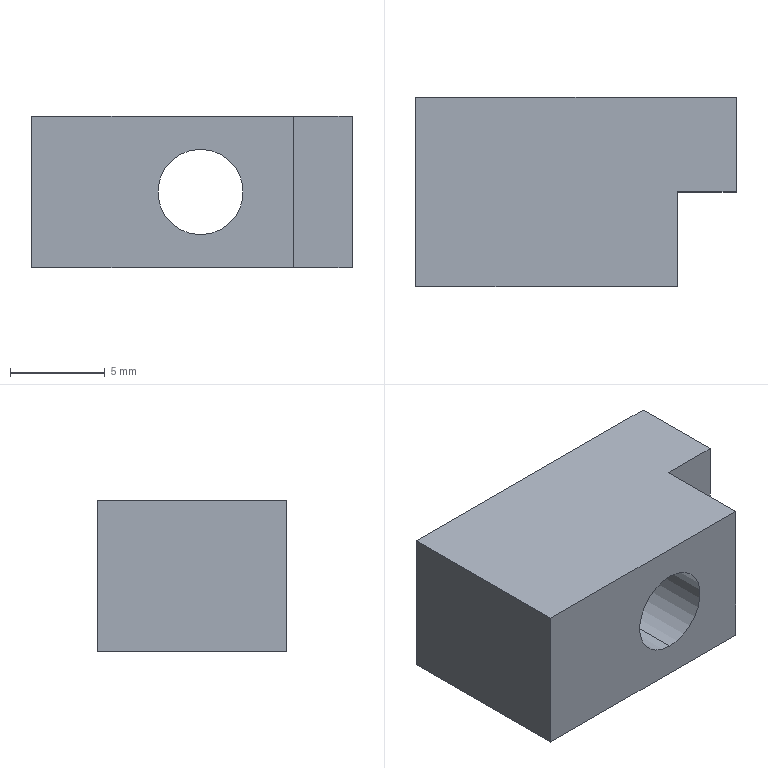Part | STEP file | Shift T-head fixing seat | 1 solid | 13 faces | box 16.9 x 10 x 8 mm | volume 941.722 mm3 | plane 9 | cylinder 4 | commonest cylinder face diameters 4.5 x2 7.5 x2
STEP:
#1=CARTESIAN_POINT('',(0.,0.,0.));
#2=DIRECTION('',(0.,0.,1.));
#3=DIRECTION('',(1.,0.,0.));
#4=AXIS2_PLACEMENT_3D('',#1,#2,#3);
#5=CARTESIAN_POINT('',(4.,5.5,7.75));
#6=VERTEX_POINT('',#5);
#7=CARTESIAN_POINT('',(4.,10.,7.75));
#8=VERTEX_POINT('',#7);
#9=CARTESIAN_POINT('',(4.,10.,7.75));
#10=DIRECTION('',(0.,1.,0.));
#11=VECTOR('',#10,1.);
#12=LINE('',#9,#11);
#13=CARTESIAN_POINT('',(4.,10.,4.));
#14=DIRECTION('',(0.,1.,0.));
#15=DIRECTION('',(0.,0.,1.));
#16=AXIS2_PLACEMENT_3D('',#13,#14,#15);
#17=CYLINDRICAL_SURFACE('',#16,3.75);
#18=CARTESIAN_POINT('',(6.283,0.));
#19=DIRECTION('',(0.,1.));
#20=VECTOR('',#19,1.);
#21=LINE('',#18,#20);
#22=(GEOMETRIC_REPRESENTATION_CONTEXT(2)PARAMETRIC_REPRESENTATION_CONTEXT()REPRESENTATION_CONTEXT('',''));
#23=DEFINITIONAL_REPRESENTATION('',(#21),#22);
#24=PCURVE('',#17,#23);
#25=CARTESIAN_POINT('',(4.,10.,4.));
#26=DIRECTION('',(0.,1.,0.));
#27=DIRECTION('',(0.,0.,1.));
#28=AXIS2_PLACEMENT_3D('',#25,#26,#27);
#29=CYLINDRICAL_SURFACE('',#28,3.75);
#30=CARTESIAN_POINT('',(0.,0.));
#31=DIRECTION('',(0.,1.));
#32=VECTOR('',#31,1.);
#33=LINE('',#30,#32);
#34=(GEOMETRIC_REPRESENTATION_CONTEXT(2)PARAMETRIC_REPRESENTATION_CONTEXT()REPRESENTATION_CONTEXT('',''));
#35=DEFINITIONAL_REPRESENTATION('',(#33),#34);
#36=PCURVE('',#29,#35);
#37=SURFACE_CURVE('',#12,(#24,#36),.PCURVE_S1.);
#38=EDGE_CURVE('',#6,#8,#37,.T.);
#39=ORIENTED_EDGE('',*,*,#38,.T.);
#40=CARTESIAN_POINT('',(4.,10.,0.25));
#41=VERTEX_POINT('',#40);
#42=CARTESIAN_POINT('',(4.,10.,4.));
#43=DIRECTION('',(0.,1.,0.));
#44=DIRECTION('',(0.,0.,1.));
#45=AXIS2_PLACEMENT_3D('',#42,#43,#44);
#46=CIRCLE('',#45,3.75);
#47=CARTESIAN_POINT('',(0.,0.));
#48=DIRECTION('',(1.,0.));
#49=VECTOR('',#48,1.);
#50=LINE('',#47,#49);
#51=(GEOMETRIC_REPRESENTATION_CONTEXT(2)PARAMETRIC_REPRESENTATION_CONTEXT()REPRESENTATION_CONTEXT('',''));
#52=DEFINITIONAL_REPRESENTATION('',(#50),#51);
#53=PCURVE('',#17,#52);
#54=CARTESIAN_POINT('',(0.,10.,8.));
#55=DIRECTION('',(0.,-1.,0.));
#56=DIRECTION('',(1.,0.,0.));
#57=AXIS2_PLACEMENT_3D('',#54,#55,#56);
#58=PLANE('',#57);
#59=CARTESIAN_POINT('',(4.,-0.25));
#60=CARTESIAN_POINT('',(10.495,-0.25));
#61=CARTESIAN_POINT('',(7.248,-5.875));
#62=CARTESIAN_POINT('',(4.,-11.5));
#63=CARTESIAN_POINT('',(0.7524,-5.875));
#64=CARTESIAN_POINT('',(-2.495,-0.25));
#65=CARTESIAN_POINT('',(4.,-0.25));
#66=(BOUNDED_CURVE()B_SPLINE_CURVE(2,(#59,#60,#61,#62,#63,#64,#65),.UNSPECIFIED.,.T.,.F.)B_SPLINE_CURVE_WITH_KNOTS((1,2,2,2,2,1),(-2.094,0.,2.094,4.189,6.283,8.378),.UNSPECIFIED.)CURVE()GEOMETRIC_REPRESENTATION_ITEM()RATIONAL_B_SPLINE_CURVE((1.,0.5,1.,0.5,1.,0.5,1.))REPRESENTATION_ITEM(''));
#67=(GEOMETRIC_REPRESENTATION_CONTEXT(2)PARAMETRIC_REPRESENTATION_CONTEXT()REPRESENTATION_CONTEXT('',''));
#68=DEFINITIONAL_REPRESENTATION('',(#66),#67);
#69=PCURVE('',#58,#68);
#70=SURFACE_CURVE('',#46,(#53,#69),.PCURVE_S1.);
#71=EDGE_CURVE('',#41,#8,#70,.T.);
#72=ORIENTED_EDGE('',*,*,#71,.F.);
#73=CARTESIAN_POINT('',(4.,5.5,0.25));
#74=VERTEX_POINT('',#73);
#75=CARTESIAN_POINT('',(4.,10.,0.25));
#76=DIRECTION('',(0.,1.,0.));
#77=VECTOR('',#76,1.);
#78=LINE('',#75,#77);
#79=CARTESIAN_POINT('',(3.142,0.));
#80=DIRECTION('',(0.,1.));
#81=VECTOR('',#80,1.);
#82=LINE('',#79,#81);
#83=(GEOMETRIC_REPRESENTATION_CONTEXT(2)PARAMETRIC_REPRESENTATION_CONTEXT()REPRESENTATION_CONTEXT('',''));
#84=DEFINITIONAL_REPRESENTATION('',(#82),#83);
#85=PCURVE('',#17,#84);
#86=CARTESIAN_POINT('',(3.142,0.));
#87=DIRECTION('',(0.,1.));
#88=VECTOR('',#87,1.);
#89=LINE('',#86,#88);
#90=(GEOMETRIC_REPRESENTATION_CONTEXT(2)PARAMETRIC_REPRESENTATION_CONTEXT()REPRESENTATION_CONTEXT('',''));
#91=DEFINITIONAL_REPRESENTATION('',(#89),#90);
#92=PCURVE('',#29,#91);
#93=SURFACE_CURVE('',#78,(#85,#92),.PCURVE_S1.);
#94=EDGE_CURVE('',#74,#41,#93,.T.);
#95=ORIENTED_EDGE('',*,*,#94,.F.);
#96=CARTESIAN_POINT('',(4.,5.5,4.));
#97=DIRECTION('',(0.,1.,0.));
#98=DIRECTION('',(0.,0.,1.));
#99=AXIS2_PLACEMENT_3D('',#96,#97,#98);
#100=CIRCLE('',#99,3.75);
#101=CARTESIAN_POINT('',(0.,-4.5));
#102=DIRECTION('',(1.,0.));
#103=VECTOR('',#102,1.);
#104=LINE('',#101,#103);
#105=(GEOMETRIC_REPRESENTATION_CONTEXT(2)PARAMETRIC_REPRESENTATION_CONTEXT()REPRESENTATION_CONTEXT('',''));
#106=DEFINITIONAL_REPRESENTATION('',(#104),#105);
#107=PCURVE('',#17,#106);
#108=CARTESIAN_POINT('',(6.25,5.5,4.));
#109=DIRECTION('',(0.,-1.,0.));
#110=DIRECTION('',(0.,0.,-1.));
#111=AXIS2_PLACEMENT_3D('',#108,#109,#110);
#112=PLANE('',#111);
#113=CARTESIAN_POINT('',(-3.75,-2.25));
#114=CARTESIAN_POINT('',(-3.75,4.245));
#115=CARTESIAN_POINT('',(1.875,0.9976));
#116=CARTESIAN_POINT('',(7.5,-2.25));
#117=CARTESIAN_POINT('',(1.875,-5.498));
#118=CARTESIAN_POINT('',(-3.75,-8.745));
#119=CARTESIAN_POINT('',(-3.75,-2.25));
#120=(BOUNDED_CURVE()B_SPLINE_CURVE(2,(#113,#114,#115,#116,#117,#118,#119),.UNSPECIFIED.,.T.,.F.)B_SPLINE_CURVE_WITH_KNOTS((1,2,2,2,2,1),(-2.094,0.,2.094,4.189,6.283,8.378),.UNSPECIFIED.)CURVE()GEOMETRIC_REPRESENTATION_ITEM()RATIONAL_B_SPLINE_CURVE((1.,0.5,1.,0.5,1.,0.5,1.))REPRESENTATION_ITEM(''));
#121=(GEOMETRIC_REPRESENTATION_CONTEXT(2)PARAMETRIC_REPRESENTATION_CONTEXT()REPRESENTATION_CONTEXT('',''));
#122=DEFINITIONAL_REPRESENTATION('',(#120),#121);
#123=PCURVE('',#112,#122);
#124=SURFACE_CURVE('',#100,(#107,#123),.PCURVE_S1.);
#125=EDGE_CURVE('',#74,#6,#124,.T.);
#126=ORIENTED_EDGE('',*,*,#125,.T.);
#127=EDGE_LOOP('',(#39,#72,#95,#126));
#128=FACE_BOUND('',#127,.F.);
#129=ADVANCED_FACE('',(#128),#17,.F.);
#130=CARTESIAN_POINT('',(4.,0.,6.25));
#131=VERTEX_POINT('',#130);
#132=CARTESIAN_POINT('',(4.,5.5,6.25));
#133=VERTEX_POINT('',#132);
#134=CARTESIAN_POINT('',(4.,10.,6.25));
#135=DIRECTION('',(0.,1.,0.));
#136=VECTOR('',#135,1.);
#137=LINE('',#134,#136);
#138=CARTESIAN_POINT('',(4.,10.,4.));
#139=DIRECTION('',(0.,1.,0.));
#140=DIRECTION('',(0.,0.,1.));
#141=AXIS2_PLACEMENT_3D('',#138,#139,#140);
#142=CYLINDRICAL_SURFACE('',#141,2.25);
#143=CARTESIAN_POINT('',(6.283,0.));
#144=DIRECTION('',(0.,1.));
#145=VECTOR('',#144,1.);
#146=LINE('',#143,#145);
#147=(GEOMETRIC_REPRESENTATION_CONTEXT(2)PARAMETRIC_REPRESENTATION_CONTEXT()REPRESENTATION_CONTEXT('',''));
#148=DEFINITIONAL_REPRESENTATION('',(#146),#147);
#149=PCURVE('',#142,#148);
#150=CARTESIAN_POINT('',(4.,10.,4.));
#151=DIRECTION('',(0.,1.,0.));
#152=DIRECTION('',(0.,0.,1.));
#153=AXIS2_PLACEMENT_3D('',#150,#151,#152);
#154=CYLINDRICAL_SURFACE('',#153,2.25);
#155=CARTESIAN_POINT('',(0.,0.));
#156=DIRECTION('',(0.,1.));
#157=VECTOR('',#156,1.);
#158=LINE('',#155,#157);
#159=(GEOMETRIC_REPRESENTATION_CONTEXT(2)PARAMETRIC_REPRESENTATION_CONTEXT()REPRESENTATION_CONTEXT('',''));
#160=DEFINITIONAL_REPRESENTATION('',(#158),#159);
#161=PCURVE('',#154,#160);
#162=SURFACE_CURVE('',#137,(#149,#161),.PCURVE_S1.);
#163=EDGE_CURVE('',#131,#133,#162,.T.);
#164=ORIENTED_EDGE('',*,*,#163,.T.);
#165=CARTESIAN_POINT('',(4.,5.5,1.75));
#166=VERTEX_POINT('',#165);
#167=CARTESIAN_POINT('',(4.,5.5,4.));
#168=DIRECTION('',(0.,1.,0.));
#169=DIRECTION('',(0.,0.,1.));
#170=AXIS2_PLACEMENT_3D('',#167,#168,#169);
#171=CIRCLE('',#170,2.25);
#172=CARTESIAN_POINT('',(0.,-4.5));
#173=DIRECTION('',(1.,0.));
#174=VECTOR('',#173,1.);
#175=LINE('',#172,#174);
#176=(GEOMETRIC_REPRESENTATION_CONTEXT(2)PARAMETRIC_REPRESENTATION_CONTEXT()REPRESENTATION_CONTEXT('',''));
#177=DEFINITIONAL_REPRESENTATION('',(#175),#176);
#178=PCURVE('',#142,#177);
#179=CARTESIAN_POINT('',(-2.25,-2.25));
#180=CARTESIAN_POINT('',(-2.25,1.647));
#181=CARTESIAN_POINT('',(1.125,-0.3014));
#182=CARTESIAN_POINT('',(4.5,-2.25));
#183=CARTESIAN_POINT('',(1.125,-4.199));
#184=CARTESIAN_POINT('',(-2.25,-6.147));
#185=CARTESIAN_POINT('',(-2.25,-2.25));
#186=(BOUNDED_CURVE()B_SPLINE_CURVE(2,(#179,#180,#181,#182,#183,#184,#185),.UNSPECIFIED.,.T.,.F.)B_SPLINE_CURVE_WITH_KNOTS((1,2,2,2,2,1),(-2.094,0.,2.094,4.189,6.283,8.378),.UNSPECIFIED.)CURVE()GEOMETRIC_REPRESENTATION_ITEM()RATIONAL_B_SPLINE_CURVE((1.,0.5,1.,0.5,1.,0.5,1.))REPRESENTATION_ITEM(''));
#187=(GEOMETRIC_REPRESENTATION_CONTEXT(2)PARAMETRIC_REPRESENTATION_CONTEXT()REPRESENTATION_CONTEXT('',''));
#188=DEFINITIONAL_REPRESENTATION('',(#186),#187);
#189=PCURVE('',#112,#188);
#190=SURFACE_CURVE('',#171,(#178,#189),.PCURVE_S1.);
#191=EDGE_CURVE('',#166,#133,#190,.T.);
#192=ORIENTED_EDGE('',*,*,#191,.F.);
#193=CARTESIAN_POINT('',(4.,0.,1.75));
#194=VERTEX_POINT('',#193);
#195=CARTESIAN_POINT('',(4.,10.,1.75));
#196=DIRECTION('',(0.,1.,0.));
#197=VECTOR('',#196,1.);
#198=LINE('',#195,#197);
#199=CARTESIAN_POINT('',(3.142,0.));
#200=DIRECTION('',(0.,1.));
#201=VECTOR('',#200,1.);
#202=LINE('',#199,#201);
#203=(GEOMETRIC_REPRESENTATION_CONTEXT(2)PARAMETRIC_REPRESENTATION_CONTEXT()REPRESENTATION_CONTEXT('',''));
#204=DEFINITIONAL_REPRESENTATION('',(#202),#203);
#205=PCURVE('',#142,#204);
#206=CARTESIAN_POINT('',(3.142,0.));
#207=DIRECTION('',(0.,1.));
#208=VECTOR('',#207,1.);
#209=LINE('',#206,#208);
#210=(GEOMETRIC_REPRESENTATION_CONTEXT(2)PARAMETRIC_REPRESENTATION_CONTEXT()REPRESENTATION_CONTEXT('',''));
#211=DEFINITIONAL_REPRESENTATION('',(#209),#210);
#212=PCURVE('',#154,#211);
#213=SURFACE_CURVE('',#198,(#205,#212),.PCURVE_S1.);
#214=EDGE_CURVE('',#194,#166,#213,.T.);
#215=ORIENTED_EDGE('',*,*,#214,.F.);
#216=CARTESIAN_POINT('',(4.,0.,4.));
#217=DIRECTION('',(0.,1.,0.));
#218=DIRECTION('',(0.,0.,1.));
#219=AXIS2_PLACEMENT_3D('',#216,#217,#218);
#220=CIRCLE('',#219,2.25);
#221=CARTESIAN_POINT('',(0.,-10.));
#222=DIRECTION('',(1.,0.));
#223=VECTOR('',#222,1.);
#224=LINE('',#221,#223);
#225=(GEOMETRIC_REPRESENTATION_CONTEXT(2)PARAMETRIC_REPRESENTATION_CONTEXT()REPRESENTATION_CONTEXT('',''));
#226=DEFINITIONAL_REPRESENTATION('',(#224),#225);
#227=PCURVE('',#142,#226);
#228=CARTESIAN_POINT('',(0.,0.,8.));
#229=DIRECTION('',(0.,1.,0.));
#230=DIRECTION('',(0.,0.,1.));
#231=AXIS2_PLACEMENT_3D('',#228,#229,#230);
#232=PLANE('',#231);
#233=CARTESIAN_POINT('',(-4.,4.));
#234=DIRECTION('',(1.,0.));
#235=AXIS2_PLACEMENT_2D('',#233,#234);
#236=CIRCLE('',#235,2.25);
#237=(GEOMETRIC_REPRESENTATION_CONTEXT(2)PARAMETRIC_REPRESENTATION_CONTEXT()REPRESENTATION_CONTEXT('',''));
#238=DEFINITIONAL_REPRESENTATION('',(#236),#237);
#239=PCURVE('',#232,#238);
#240=SURFACE_CURVE('',#220,(#227,#239),.PCURVE_S1.);
#241=EDGE_CURVE('',#194,#131,#240,.T.);
#242=ORIENTED_EDGE('',*,*,#241,.T.);
#243=EDGE_LOOP('',(#164,#192,#215,#242));
#244=FACE_BOUND('',#243,.F.);
#245=ADVANCED_FACE('',(#244),#142,.F.);
#246=CARTESIAN_POINT('',(-4.9,10.,0.));
#247=VERTEX_POINT('',#246);
#248=CARTESIAN_POINT('',(-4.9,0.,0.));
#249=VERTEX_POINT('',#248);
#250=CARTESIAN_POINT('',(-4.9,10.,0.));
#251=DIRECTION('',(0.,-1.,0.));
#252=VECTOR('',#251,1.);
#253=LINE('',#250,#252);
#254=CARTESIAN_POINT('',(-4.9,0.,8.));
#255=DIRECTION('',(1.,0.,0.));
#256=DIRECTION('',(0.,0.,-1.));
#257=AXIS2_PLACEMENT_3D('',#254,#255,#256);
#258=PLANE('',#257);
#259=CARTESIAN_POINT('',(8.,10.));
#260=DIRECTION('',(0.,-1.));
#261=VECTOR('',#260,1.);
#262=LINE('',#259,#261);
#263=(GEOMETRIC_REPRESENTATION_CONTEXT(2)PARAMETRIC_REPRESENTATION_CONTEXT()REPRESENTATION_CONTEXT('',''));
#264=DEFINITIONAL_REPRESENTATION('',(#262),#263);
#265=PCURVE('',#258,#264);
#266=CARTESIAN_POINT('',(0.,10.,0.));
#267=DIRECTION('',(0.,0.,-1.));
#268=DIRECTION('',(-1.,0.,0.));
#269=AXIS2_PLACEMENT_3D('',#266,#267,#268);
#270=PLANE('',#269);
#271=CARTESIAN_POINT('',(4.9,0.));
#272=DIRECTION('',(0.,-1.));
#273=VECTOR('',#272,1.);
#274=LINE('',#271,#273);
#275=(GEOMETRIC_REPRESENTATION_CONTEXT(2)PARAMETRIC_REPRESENTATION_CONTEXT()REPRESENTATION_CONTEXT('',''));
#276=DEFINITIONAL_REPRESENTATION('',(#274),#275);
#277=PCURVE('',#270,#276);
#278=SURFACE_CURVE('',#253,(#265,#277),.PCURVE_S1.);
#279=EDGE_CURVE('',#247,#249,#278,.T.);
#280=ORIENTED_EDGE('',*,*,#279,.T.);
#281=CARTESIAN_POINT('',(-4.9,0.,8.));
#282=VERTEX_POINT('',#281);
#283=CARTESIAN_POINT('',(-4.9,0.,8.));
#284=DIRECTION('',(0.,0.,-1.));
#285=VECTOR('',#284,1.);
#286=LINE('',#283,#285);
#287=CARTESIAN_POINT('',(0.,0.));
#288=DIRECTION('',(1.,0.));
#289=VECTOR('',#288,1.);
#290=LINE('',#287,#289);
#291=(GEOMETRIC_REPRESENTATION_CONTEXT(2)PARAMETRIC_REPRESENTATION_CONTEXT()REPRESENTATION_CONTEXT('',''));
#292=DEFINITIONAL_REPRESENTATION('',(#290),#291);
#293=PCURVE('',#258,#292);
#294=CARTESIAN_POINT('',(0.,-4.9));
#295=DIRECTION('',(-1.,0.));
#296=VECTOR('',#295,1.);
#297=LINE('',#294,#296);
#298=(GEOMETRIC_REPRESENTATION_CONTEXT(2)PARAMETRIC_REPRESENTATION_CONTEXT()REPRESENTATION_CONTEXT('',''));
#299=DEFINITIONAL_REPRESENTATION('',(#297),#298);
#300=PCURVE('',#232,#299);
#301=SURFACE_CURVE('',#286,(#293,#300),.PCURVE_S1.);
#302=EDGE_CURVE('',#282,#249,#301,.T.);
#303=ORIENTED_EDGE('',*,*,#302,.F.);
#304=CARTESIAN_POINT('',(-4.9,10.,8.));
#305=VERTEX_POINT('',#304);
#306=CARTESIAN_POINT('',(-4.9,10.,8.));
#307=DIRECTION('',(0.,-1.,0.));
#308=VECTOR('',#307,1.);
#309=LINE('',#306,#308);
#310=CARTESIAN_POINT('',(0.,10.));
#311=DIRECTION('',(0.,-1.));
#312=VECTOR('',#311,1.);
#313=LINE('',#310,#312);
#314=(GEOMETRIC_REPRESENTATION_CONTEXT(2)PARAMETRIC_REPRESENTATION_CONTEXT()REPRESENTATION_CONTEXT('',''));
#315=DEFINITIONAL_REPRESENTATION('',(#313),#314);
#316=PCURVE('',#258,#315);
#317=CARTESIAN_POINT('',(0.,10.,8.));
#318=DIRECTION('',(0.,0.,-1.));
#319=DIRECTION('',(-1.,0.,0.));
#320=AXIS2_PLACEMENT_3D('',#317,#318,#319);
#321=PLANE('',#320);
#322=CARTESIAN_POINT('',(4.9,0.));
#323=DIRECTION('',(0.,-1.));
#324=VECTOR('',#323,1.);
#325=LINE('',#322,#324);
#326=(GEOMETRIC_REPRESENTATION_CONTEXT(2)PARAMETRIC_REPRESENTATION_CONTEXT()REPRESENTATION_CONTEXT('',''));
#327=DEFINITIONAL_REPRESENTATION('',(#325),#326);
#328=PCURVE('',#321,#327);
#329=SURFACE_CURVE('',#309,(#316,#328),.PCURVE_S1.);
#330=EDGE_CURVE('',#305,#282,#329,.T.);
#331=ORIENTED_EDGE('',*,*,#330,.F.);
#332=CARTESIAN_POINT('',(-4.9,10.,8.));
#333=DIRECTION('',(0.,0.,-1.));
#334=VECTOR('',#333,1.);
#335=LINE('',#332,#334);
#336=CARTESIAN_POINT('',(0.,10.));
#337=DIRECTION('',(1.,0.));
#338=VECTOR('',#337,1.);
#339=LINE('',#336,#338);
#340=(GEOMETRIC_REPRESENTATION_CONTEXT(2)PARAMETRIC_REPRESENTATION_CONTEXT()REPRESENTATION_CONTEXT('',''));
#341=DEFINITIONAL_REPRESENTATION('',(#339),#340);
#342=PCURVE('',#258,#341);
#343=CARTESIAN_POINT('',(-4.9,0.));
#344=DIRECTION('',(0.,-1.));
#345=VECTOR('',#344,1.);
#346=LINE('',#343,#345);
#347=(GEOMETRIC_REPRESENTATION_CONTEXT(2)PARAMETRIC_REPRESENTATION_CONTEXT()REPRESENTATION_CONTEXT('',''));
#348=DEFINITIONAL_REPRESENTATION('',(#346),#347);
#349=PCURVE('',#58,#348);
#350=SURFACE_CURVE('',#335,(#342,#349),.PCURVE_S1.);
#351=EDGE_CURVE('',#305,#247,#350,.T.);
#352=ORIENTED_EDGE('',*,*,#351,.T.);
#353=EDGE_LOOP('',(#280,#303,#331,#352));
#354=FACE_BOUND('',#353,.T.);
#355=ADVANCED_FACE('',(#354),#258,.F.);
#356=CARTESIAN_POINT('',(4.,0.,4.));
#357=DIRECTION('',(0.,1.,0.));
#358=DIRECTION('',(0.,0.,1.));
#359=AXIS2_PLACEMENT_3D('',#356,#357,#358);
#360=CIRCLE('',#359,2.25);
#361=CARTESIAN_POINT('',(-4.,4.));
#362=DIRECTION('',(1.,0.));
#363=AXIS2_PLACEMENT_2D('',#361,#362);
#364=CIRCLE('',#363,2.25);
#365=(GEOMETRIC_REPRESENTATION_CONTEXT(2)PARAMETRIC_REPRESENTATION_CONTEXT()REPRESENTATION_CONTEXT('',''));
#366=DEFINITIONAL_REPRESENTATION('',(#364),#365);
#367=PCURVE('',#232,#366);
#368=CARTESIAN_POINT('',(0.,-10.));
#369=DIRECTION('',(1.,0.));
#370=VECTOR('',#369,1.);
#371=LINE('',#368,#370);
#372=(GEOMETRIC_REPRESENTATION_CONTEXT(2)PARAMETRIC_REPRESENTATION_CONTEXT()REPRESENTATION_CONTEXT('',''));
#373=DEFINITIONAL_REPRESENTATION('',(#371),#372);
#374=PCURVE('',#154,#373);
#375=SURFACE_CURVE('',#360,(#367,#374),.PCURVE_S1.);
#376=EDGE_CURVE('',#131,#194,#375,.T.);
#377=ORIENTED_EDGE('',*,*,#376,.T.);
#378=ORIENTED_EDGE('',*,*,#241,.T.);
#379=EDGE_LOOP('',(#377,#378));
#380=FACE_BOUND('',#379,.T.);
#381=CARTESIAN_POINT('',(8.9,0.,0.));
#382=VERTEX_POINT('',#381);
#383=CARTESIAN_POINT('',(0.,0.,0.));
#384=DIRECTION('',(1.,0.,0.));
#385=VECTOR('',#384,1.);
#386=LINE('',#383,#385);
#387=CARTESIAN_POINT('',(-8.,0.));
#388=DIRECTION('',(0.,1.));
#389=VECTOR('',#388,1.);
#390=LINE('',#387,#389);
#391=(GEOMETRIC_REPRESENTATION_CONTEXT(2)PARAMETRIC_REPRESENTATION_CONTEXT()REPRESENTATION_CONTEXT('',''));
#392=DEFINITIONAL_REPRESENTATION('',(#390),#391);
#393=PCURVE('',#232,#392);
#394=CARTESIAN_POINT('',(0.,-10.));
#395=DIRECTION('',(-1.,0.));
#396=VECTOR('',#395,1.);
#397=LINE('',#394,#396);
#398=(GEOMETRIC_REPRESENTATION_CONTEXT(2)PARAMETRIC_REPRESENTATION_CONTEXT()REPRESENTATION_CONTEXT('',''));
#399=DEFINITIONAL_REPRESENTATION('',(#397),#398);
#400=PCURVE('',#270,#399);
#401=SURFACE_CURVE('',#386,(#393,#400),.PCURVE_S1.);
#402=EDGE_CURVE('',#249,#382,#401,.T.);
#403=ORIENTED_EDGE('',*,*,#402,.T.);
#404=CARTESIAN_POINT('',(8.9,0.,8.));
#405=VERTEX_POINT('',#404);
#406=CARTESIAN_POINT('',(8.9,0.,8.));
#407=DIRECTION('',(0.,0.,1.));
#408=VECTOR('',#407,1.);
#409=LINE('',#406,#408);
#410=CARTESIAN_POINT('',(0.,8.9));
#411=DIRECTION('',(1.,0.));
#412=VECTOR('',#411,1.);
#413=LINE('',#410,#412);
#414=(GEOMETRIC_REPRESENTATION_CONTEXT(2)PARAMETRIC_REPRESENTATION_CONTEXT()REPRESENTATION_CONTEXT('',''));
#415=DEFINITIONAL_REPRESENTATION('',(#413),#414);
#416=PCURVE('',#232,#415);
#417=CARTESIAN_POINT('',(8.9,5.,0.));
#418=DIRECTION('',(-1.,0.,0.));
#419=DIRECTION('',(0.,-1.,0.));
#420=AXIS2_PLACEMENT_3D('',#417,#418,#419);
#421=PLANE('',#420);
#422=CARTESIAN_POINT('',(5.,8.));
#423=DIRECTION('',(0.,1.));
#424=VECTOR('',#423,1.);
#425=LINE('',#422,#424);
#426=(GEOMETRIC_REPRESENTATION_CONTEXT(2)PARAMETRIC_REPRESENTATION_CONTEXT()REPRESENTATION_CONTEXT('',''));
#427=DEFINITIONAL_REPRESENTATION('',(#425),#426);
#428=PCURVE('',#421,#427);
#429=SURFACE_CURVE('',#409,(#416,#428),.PCURVE_S1.);
#430=EDGE_CURVE('',#382,#405,#429,.T.);
#431=ORIENTED_EDGE('',*,*,#430,.T.);
#432=CARTESIAN_POINT('',(0.,0.,8.));
#433=DIRECTION('',(1.,0.,0.));
#434=VECTOR('',#433,1.);
#435=LINE('',#432,#434);
#436=CARTESIAN_POINT('',(0.,0.));
#437=DIRECTION('',(0.,1.));
#438=VECTOR('',#437,1.);
#439=LINE('',#436,#438);
#440=(GEOMETRIC_REPRESENTATION_CONTEXT(2)PARAMETRIC_REPRESENTATION_CONTEXT()REPRESENTATION_CONTEXT('',''));
#441=DEFINITIONAL_REPRESENTATION('',(#439),#440);
#442=PCURVE('',#232,#441);
#443=CARTESIAN_POINT('',(0.,-10.));
#444=DIRECTION('',(-1.,0.));
#445=VECTOR('',#444,1.);
#446=LINE('',#443,#445);
#447=(GEOMETRIC_REPRESENTATION_CONTEXT(2)PARAMETRIC_REPRESENTATION_CONTEXT()REPRESENTATION_CONTEXT('',''));
#448=DEFINITIONAL_REPRESENTATION('',(#446),#447);
#449=PCURVE('',#321,#448);
#450=SURFACE_CURVE('',#435,(#442,#449),.PCURVE_S1.);
#451=EDGE_CURVE('',#282,#405,#450,.T.);
#452=ORIENTED_EDGE('',*,*,#451,.F.);
#453=ORIENTED_EDGE('',*,*,#302,.T.);
#454=EDGE_LOOP('',(#403,#431,#452,#453));
#455=FACE_BOUND('',#454,.T.);
#456=ADVANCED_FACE('',(#380,#455),#232,.F.);
#457=CARTESIAN_POINT('',(12.,5.,8.));
#458=VERTEX_POINT('',#457);
#459=CARTESIAN_POINT('',(12.,10.,8.));
#460=VERTEX_POINT('',#459);
#461=CARTESIAN_POINT('',(12.,0.,8.));
#462=DIRECTION('',(0.,1.,0.));
#463=VECTOR('',#462,1.);
#464=LINE('',#461,#463);
#465=CARTESIAN_POINT('',(12.,0.,8.));
#466=DIRECTION('',(-1.,0.,0.));
#467=DIRECTION('',(0.,0.,1.));
#468=AXIS2_PLACEMENT_3D('',#465,#466,#467);
#469=PLANE('',#468);
#470=CARTESIAN_POINT('',(0.,0.));
#471=DIRECTION('',(0.,1.));
#472=VECTOR('',#471,1.);
#473=LINE('',#470,#472);
#474=(GEOMETRIC_REPRESENTATION_CONTEXT(2)PARAMETRIC_REPRESENTATION_CONTEXT()REPRESENTATION_CONTEXT('',''));
#475=DEFINITIONAL_REPRESENTATION('',(#473),#474);
#476=PCURVE('',#469,#475);
#477=CARTESIAN_POINT('',(-12.,-10.));
#478=DIRECTION('',(0.,1.));
#479=VECTOR('',#478,1.);
#480=LINE('',#477,#479);
#481=(GEOMETRIC_REPRESENTATION_CONTEXT(2)PARAMETRIC_REPRESENTATION_CONTEXT()REPRESENTATION_CONTEXT('',''));
#482=DEFINITIONAL_REPRESENTATION('',(#480),#481);
#483=PCURVE('',#321,#482);
#484=SURFACE_CURVE('',#464,(#476,#483),.PCURVE_S1.);
#485=EDGE_CURVE('',#458,#460,#484,.T.);
#486=ORIENTED_EDGE('',*,*,#485,.F.);
#487=CARTESIAN_POINT('',(12.,5.,0.));
#488=VERTEX_POINT('',#487);
#489=CARTESIAN_POINT('',(12.,5.,8.));
#490=DIRECTION('',(0.,0.,-1.));
#491=VECTOR('',#490,1.);
#492=LINE('',#489,#491);
#493=CARTESIAN_POINT('',(0.,5.));
#494=DIRECTION('',(-1.,0.));
#495=VECTOR('',#494,1.);
#496=LINE('',#493,#495);
#497=(GEOMETRIC_REPRESENTATION_CONTEXT(2)PARAMETRIC_REPRESENTATION_CONTEXT()REPRESENTATION_CONTEXT('',''));
#498=DEFINITIONAL_REPRESENTATION('',(#496),#497);
#499=PCURVE('',#469,#498);
#500=CARTESIAN_POINT('',(24.425,5.,0.));
#501=DIRECTION('',(0.,1.,0.));
#502=DIRECTION('',(-1.,0.,0.));
#503=AXIS2_PLACEMENT_3D('',#500,#501,#502);
#504=PLANE('',#503);
#505=CARTESIAN_POINT('',(12.425,8.));
#506=DIRECTION('',(0.,-1.));
#507=VECTOR('',#506,1.);
#508=LINE('',#505,#507);
#509=(GEOMETRIC_REPRESENTATION_CONTEXT(2)PARAMETRIC_REPRESENTATION_CONTEXT()REPRESENTATION_CONTEXT('',''));
#510=DEFINITIONAL_REPRESENTATION('',(#508),#509);
#511=PCURVE('',#504,#510);
#512=SURFACE_CURVE('',#492,(#499,#511),.PCURVE_S1.);
#513=EDGE_CURVE('',#458,#488,#512,.T.);
#514=ORIENTED_EDGE('',*,*,#513,.T.);
#515=CARTESIAN_POINT('',(12.,10.,0.));
#516=VERTEX_POINT('',#515);
#517=CARTESIAN_POINT('',(12.,0.,0.));
#518=DIRECTION('',(0.,1.,0.));
#519=VECTOR('',#518,1.);
#520=LINE('',#517,#519);
#521=CARTESIAN_POINT('',(-8.,0.));
#522=DIRECTION('',(0.,1.));
#523=VECTOR('',#522,1.);
#524=LINE('',#521,#523);
#525=(GEOMETRIC_REPRESENTATION_CONTEXT(2)PARAMETRIC_REPRESENTATION_CONTEXT()REPRESENTATION_CONTEXT('',''));
#526=DEFINITIONAL_REPRESENTATION('',(#524),#525);
#527=PCURVE('',#469,#526);
#528=CARTESIAN_POINT('',(-12.,-10.));
#529=DIRECTION('',(0.,1.));
#530=VECTOR('',#529,1.);
#531=LINE('',#528,#530);
#532=(GEOMETRIC_REPRESENTATION_CONTEXT(2)PARAMETRIC_REPRESENTATION_CONTEXT()REPRESENTATION_CONTEXT('',''));
#533=DEFINITIONAL_REPRESENTATION('',(#531),#532);
#534=PCURVE('',#270,#533);
#535=SURFACE_CURVE('',#520,(#527,#534),.PCURVE_S1.);
#536=EDGE_CURVE('',#488,#516,#535,.T.);
#537=ORIENTED_EDGE('',*,*,#536,.T.);
#538=CARTESIAN_POINT('',(12.,10.,8.));
#539=DIRECTION('',(0.,0.,-1.));
#540=VECTOR('',#539,1.);
#541=LINE('',#538,#540);
#542=CARTESIAN_POINT('',(0.,10.));
#543=DIRECTION('',(-1.,0.));
#544=VECTOR('',#543,1.);
#545=LINE('',#542,#544);
#546=(GEOMETRIC_REPRESENTATION_CONTEXT(2)PARAMETRIC_REPRESENTATION_CONTEXT()REPRESENTATION_CONTEXT('',''));
#547=DEFINITIONAL_REPRESENTATION('',(#545),#546);
#548=PCURVE('',#469,#547);
#549=CARTESIAN_POINT('',(12.,0.));
#550=DIRECTION('',(0.,-1.));
#551=VECTOR('',#550,1.);
#552=LINE('',#549,#551);
#553=(GEOMETRIC_REPRESENTATION_CONTEXT(2)PARAMETRIC_REPRESENTATION_CONTEXT()REPRESENTATION_CONTEXT('',''));
#554=DEFINITIONAL_REPRESENTATION('',(#552),#553);
#555=PCURVE('',#58,#554);
#556=SURFACE_CURVE('',#541,(#548,#555),.PCURVE_S1.);
#557=EDGE_CURVE('',#460,#516,#556,.T.);
#558=ORIENTED_EDGE('',*,*,#557,.F.);
#559=EDGE_LOOP('',(#486,#514,#537,#558));
#560=FACE_BOUND('',#559,.T.);
#561=ADVANCED_FACE('',(#560),#469,.F.);
#562=CARTESIAN_POINT('',(4.,10.,4.));
#563=DIRECTION('',(0.,1.,0.));
#564=DIRECTION('',(0.,0.,1.));
#565=AXIS2_PLACEMENT_3D('',#562,#563,#564);
#566=CIRCLE('',#565,3.75);
#567=CARTESIAN_POINT('',(4.,-0.25));
#568=CARTESIAN_POINT('',(10.495,-0.25));
#569=CARTESIAN_POINT('',(7.248,-5.875));
#570=CARTESIAN_POINT('',(4.,-11.5));
#571=CARTESIAN_POINT('',(0.7524,-5.875));
#572=CARTESIAN_POINT('',(-2.495,-0.25));
#573=CARTESIAN_POINT('',(4.,-0.25));
#574=(BOUNDED_CURVE()B_SPLINE_CURVE(2,(#567,#568,#569,#570,#571,#572,#573),.UNSPECIFIED.,.T.,.F.)B_SPLINE_CURVE_WITH_KNOTS((1,2,2,2,2,1),(-2.094,0.,2.094,4.189,6.283,8.378),.UNSPECIFIED.)CURVE()GEOMETRIC_REPRESENTATION_ITEM()RATIONAL_B_SPLINE_CURVE((1.,0.5,1.,0.5,1.,0.5,1.))REPRESENTATION_ITEM(''));
#575=(GEOMETRIC_REPRESENTATION_CONTEXT(2)PARAMETRIC_REPRESENTATION_CONTEXT()REPRESENTATION_CONTEXT('',''));
#576=DEFINITIONAL_REPRESENTATION('',(#574),#575);
#577=PCURVE('',#58,#576);
#578=CARTESIAN_POINT('',(0.,0.));
#579=DIRECTION('',(1.,0.));
#580=VECTOR('',#579,1.);
#581=LINE('',#578,#580);
#582=(GEOMETRIC_REPRESENTATION_CONTEXT(2)PARAMETRIC_REPRESENTATION_CONTEXT()REPRESENTATION_CONTEXT('',''));
#583=DEFINITIONAL_REPRESENTATION('',(#581),#582);
#584=PCURVE('',#29,#583);
#585=SURFACE_CURVE('',#566,(#577,#584),.PCURVE_S1.);
#586=EDGE_CURVE('',#8,#41,#585,.T.);
#587=ORIENTED_EDGE('',*,*,#586,.F.);
#588=ORIENTED_EDGE('',*,*,#71,.F.);
#589=EDGE_LOOP('',(#587,#588));
#590=FACE_BOUND('',#589,.T.);
#591=CARTESIAN_POINT('',(0.,10.,0.));
#592=DIRECTION('',(-1.,0.,0.));
#593=VECTOR('',#592,1.);
#594=LINE('',#591,#593);
#595=CARTESIAN_POINT('',(0.,-8.));
#596=DIRECTION('',(-1.,0.));
#597=VECTOR('',#596,1.);
#598=LINE('',#595,#597);
#599=(GEOMETRIC_REPRESENTATION_CONTEXT(2)PARAMETRIC_REPRESENTATION_CONTEXT()REPRESENTATION_CONTEXT('',''));
#600=DEFINITIONAL_REPRESENTATION('',(#598),#599);
#601=PCURVE('',#58,#600);
#602=CARTESIAN_POINT('',(0.,0.));
#603=DIRECTION('',(1.,0.));
#604=VECTOR('',#603,1.);
#605=LINE('',#602,#604);
#606=(GEOMETRIC_REPRESENTATION_CONTEXT(2)PARAMETRIC_REPRESENTATION_CONTEXT()REPRESENTATION_CONTEXT('',''));
#607=DEFINITIONAL_REPRESENTATION('',(#605),#606);
#608=PCURVE('',#270,#607);
#609=SURFACE_CURVE('',#594,(#601,#608),.PCURVE_S1.);
#610=EDGE_CURVE('',#516,#247,#609,.T.);
#611=ORIENTED_EDGE('',*,*,#610,.T.);
#612=ORIENTED_EDGE('',*,*,#351,.F.);
#613=CARTESIAN_POINT('',(0.,10.,8.));
#614=DIRECTION('',(-1.,0.,0.));
#615=VECTOR('',#614,1.);
#616=LINE('',#613,#615);
#617=CARTESIAN_POINT('',(0.,0.));
#618=DIRECTION('',(-1.,0.));
#619=VECTOR('',#618,1.);
#620=LINE('',#617,#619);
#621=(GEOMETRIC_REPRESENTATION_CONTEXT(2)PARAMETRIC_REPRESENTATION_CONTEXT()REPRESENTATION_CONTEXT('',''));
#622=DEFINITIONAL_REPRESENTATION('',(#620),#621);
#623=PCURVE('',#58,#622);
#624=CARTESIAN_POINT('',(0.,0.));
#625=DIRECTION('',(1.,0.));
#626=VECTOR('',#625,1.);
#627=LINE('',#624,#626);
#628=(GEOMETRIC_REPRESENTATION_CONTEXT(2)PARAMETRIC_REPRESENTATION_CONTEXT()REPRESENTATION_CONTEXT('',''));
#629=DEFINITIONAL_REPRESENTATION('',(#627),#628);
#630=PCURVE('',#321,#629);
#631=SURFACE_CURVE('',#616,(#623,#630),.PCURVE_S1.);
#632=EDGE_CURVE('',#460,#305,#631,.T.);
#633=ORIENTED_EDGE('',*,*,#632,.F.);
#634=ORIENTED_EDGE('',*,*,#557,.T.);
#635=EDGE_LOOP('',(#611,#612,#633,#634));
#636=FACE_BOUND('',#635,.T.);
#637=ADVANCED_FACE('',(#590,#636),#58,.F.);
#638=ORIENTED_EDGE('',*,*,#451,.T.);
#639=CARTESIAN_POINT('',(8.9,5.,8.));
#640=VERTEX_POINT('',#639);
#641=CARTESIAN_POINT('',(8.9,5.,8.));
#642=DIRECTION('',(0.,-1.,0.));
#643=VECTOR('',#642,1.);
#644=LINE('',#641,#643);
#645=CARTESIAN_POINT('',(-8.9,-5.));
#646=DIRECTION('',(0.,-1.));
#647=VECTOR('',#646,1.);
#648=LINE('',#645,#647);
#649=(GEOMETRIC_REPRESENTATION_CONTEXT(2)PARAMETRIC_REPRESENTATION_CONTEXT()REPRESENTATION_CONTEXT('',''));
#650=DEFINITIONAL_REPRESENTATION('',(#648),#649);
#651=PCURVE('',#321,#650);
#652=CARTESIAN_POINT('',(0.,8.));
#653=DIRECTION('',(1.,0.));
#654=VECTOR('',#653,1.);
#655=LINE('',#652,#654);
#656=(GEOMETRIC_REPRESENTATION_CONTEXT(2)PARAMETRIC_REPRESENTATION_CONTEXT()REPRESENTATION_CONTEXT('',''));
#657=DEFINITIONAL_REPRESENTATION('',(#655),#656);
#658=PCURVE('',#421,#657);
#659=SURFACE_CURVE('',#644,(#651,#658),.PCURVE_S1.);
#660=EDGE_CURVE('',#640,#405,#659,.T.);
#661=ORIENTED_EDGE('',*,*,#660,.F.);
#662=CARTESIAN_POINT('',(24.425,5.,8.));
#663=DIRECTION('',(-1.,0.,0.));
#664=VECTOR('',#663,1.);
#665=LINE('',#662,#664);
#666=CARTESIAN_POINT('',(-24.425,-5.));
#667=DIRECTION('',(1.,0.));
#668=VECTOR('',#667,1.);
#669=LINE('',#666,#668);
#670=(GEOMETRIC_REPRESENTATION_CONTEXT(2)PARAMETRIC_REPRESENTATION_CONTEXT()REPRESENTATION_CONTEXT('',''));
#671=DEFINITIONAL_REPRESENTATION('',(#669),#670);
#672=PCURVE('',#321,#671);
#673=CARTESIAN_POINT('',(0.,8.));
#674=DIRECTION('',(1.,0.));
#675=VECTOR('',#674,1.);
#676=LINE('',#673,#675);
#677=(GEOMETRIC_REPRESENTATION_CONTEXT(2)PARAMETRIC_REPRESENTATION_CONTEXT()REPRESENTATION_CONTEXT('',''));
#678=DEFINITIONAL_REPRESENTATION('',(#676),#677);
#679=PCURVE('',#504,#678);
#680=SURFACE_CURVE('',#665,(#672,#679),.PCURVE_S1.);
#681=EDGE_CURVE('',#458,#640,#680,.T.);
#682=ORIENTED_EDGE('',*,*,#681,.F.);
#683=ORIENTED_EDGE('',*,*,#485,.T.);
#684=ORIENTED_EDGE('',*,*,#632,.T.);
#685=ORIENTED_EDGE('',*,*,#330,.T.);
#686=EDGE_LOOP('',(#638,#661,#682,#683,#684,#685));
#687=FACE_BOUND('',#686,.T.);
#688=ADVANCED_FACE('',(#687),#321,.F.);
#689=CARTESIAN_POINT('',(8.9,5.,0.));
#690=VERTEX_POINT('',#689);
#691=CARTESIAN_POINT('',(8.9,5.,0.));
#692=DIRECTION('',(0.,-1.,0.));
#693=VECTOR('',#692,1.);
#694=LINE('',#691,#693);
#695=CARTESIAN_POINT('',(-8.9,-5.));
#696=DIRECTION('',(0.,-1.));
#697=VECTOR('',#696,1.);
#698=LINE('',#695,#697);
#699=(GEOMETRIC_REPRESENTATION_CONTEXT(2)PARAMETRIC_REPRESENTATION_CONTEXT()REPRESENTATION_CONTEXT('',''));
#700=DEFINITIONAL_REPRESENTATION('',(#698),#699);
#701=PCURVE('',#270,#700);
#702=CARTESIAN_POINT('',(0.,0.));
#703=DIRECTION('',(1.,0.));
#704=VECTOR('',#703,1.);
#705=LINE('',#702,#704);
#706=(GEOMETRIC_REPRESENTATION_CONTEXT(2)PARAMETRIC_REPRESENTATION_CONTEXT()REPRESENTATION_CONTEXT('',''));
#707=DEFINITIONAL_REPRESENTATION('',(#705),#706);
#708=PCURVE('',#421,#707);
#709=SURFACE_CURVE('',#694,(#701,#708),.PCURVE_S1.);
#710=EDGE_CURVE('',#690,#382,#709,.T.);
#711=ORIENTED_EDGE('',*,*,#710,.T.);
#712=ORIENTED_EDGE('',*,*,#402,.F.);
#713=ORIENTED_EDGE('',*,*,#279,.F.);
#714=ORIENTED_EDGE('',*,*,#610,.F.);
#715=ORIENTED_EDGE('',*,*,#536,.F.);
#716=CARTESIAN_POINT('',(0.,5.,0.));
#717=DIRECTION('',(1.,0.,0.));
#718=VECTOR('',#717,1.);
#719=LINE('',#716,#718);
#720=CARTESIAN_POINT('',(0.,-5.));
#721=DIRECTION('',(-1.,0.));
#722=VECTOR('',#721,1.);
#723=LINE('',#720,#722);
#724=(GEOMETRIC_REPRESENTATION_CONTEXT(2)PARAMETRIC_REPRESENTATION_CONTEXT()REPRESENTATION_CONTEXT('',''));
#725=DEFINITIONAL_REPRESENTATION('',(#723),#724);
#726=PCURVE('',#270,#725);
#727=CARTESIAN_POINT('',(24.425,0.));
#728=DIRECTION('',(-1.,0.));
#729=VECTOR('',#728,1.);
#730=LINE('',#727,#729);
#731=(GEOMETRIC_REPRESENTATION_CONTEXT(2)PARAMETRIC_REPRESENTATION_CONTEXT()REPRESENTATION_CONTEXT('',''));
#732=DEFINITIONAL_REPRESENTATION('',(#730),#731);
#733=PCURVE('',#504,#732);
#734=SURFACE_CURVE('',#719,(#726,#733),.PCURVE_S1.);
#735=EDGE_CURVE('',#690,#488,#734,.T.);
#736=ORIENTED_EDGE('',*,*,#735,.F.);
#737=EDGE_LOOP('',(#711,#712,#713,#714,#715,#736));
#738=FACE_BOUND('',#737,.T.);
#739=ADVANCED_FACE('',(#738),#270,.T.);
#740=ORIENTED_EDGE('',*,*,#710,.F.);
#741=CARTESIAN_POINT('',(8.9,5.,0.));
#742=DIRECTION('',(0.,0.,1.));
#743=VECTOR('',#742,1.);
#744=LINE('',#741,#743);
#745=CARTESIAN_POINT('',(0.,0.));
#746=DIRECTION('',(0.,1.));
#747=VECTOR('',#746,1.);
#748=LINE('',#745,#747);
#749=(GEOMETRIC_REPRESENTATION_CONTEXT(2)PARAMETRIC_REPRESENTATION_CONTEXT()REPRESENTATION_CONTEXT('',''));
#750=DEFINITIONAL_REPRESENTATION('',(#748),#749);
#751=PCURVE('',#421,#750);
#752=CARTESIAN_POINT('',(15.525,0.));
#753=DIRECTION('',(0.,1.));
#754=VECTOR('',#753,1.);
#755=LINE('',#752,#754);
#756=(GEOMETRIC_REPRESENTATION_CONTEXT(2)PARAMETRIC_REPRESENTATION_CONTEXT()REPRESENTATION_CONTEXT('',''));
#757=DEFINITIONAL_REPRESENTATION('',(#755),#756);
#758=PCURVE('',#504,#757);
#759=SURFACE_CURVE('',#744,(#751,#758),.PCURVE_S1.);
#760=EDGE_CURVE('',#690,#640,#759,.T.);
#761=ORIENTED_EDGE('',*,*,#760,.T.);
#762=ORIENTED_EDGE('',*,*,#660,.T.);
#763=ORIENTED_EDGE('',*,*,#430,.F.);
#764=EDGE_LOOP('',(#740,#761,#762,#763));
#765=FACE_BOUND('',#764,.T.);
#766=ADVANCED_FACE('',(#765),#421,.F.);
#767=ORIENTED_EDGE('',*,*,#681,.T.);
#768=ORIENTED_EDGE('',*,*,#760,.F.);
#769=ORIENTED_EDGE('',*,*,#735,.T.);
#770=ORIENTED_EDGE('',*,*,#513,.F.);
#771=EDGE_LOOP('',(#767,#768,#769,#770));
#772=FACE_BOUND('',#771,.T.);
#773=ADVANCED_FACE('',(#772),#504,.F.);
#774=CARTESIAN_POINT('',(4.,5.5,4.));
#775=DIRECTION('',(0.,1.,0.));
#776=DIRECTION('',(0.,0.,1.));
#777=AXIS2_PLACEMENT_3D('',#774,#775,#776);
#778=CIRCLE('',#777,2.25);
#779=CARTESIAN_POINT('',(0.,-4.5));
#780=DIRECTION('',(1.,0.));
#781=VECTOR('',#780,1.);
#782=LINE('',#779,#781);
#783=(GEOMETRIC_REPRESENTATION_CONTEXT(2)PARAMETRIC_REPRESENTATION_CONTEXT()REPRESENTATION_CONTEXT('',''));
#784=DEFINITIONAL_REPRESENTATION('',(#782),#783);
#785=PCURVE('',#154,#784);
#786=CARTESIAN_POINT('',(-2.25,-2.25));
#787=CARTESIAN_POINT('',(-2.25,1.647));
#788=CARTESIAN_POINT('',(1.125,-0.3014));
#789=CARTESIAN_POINT('',(4.5,-2.25));
#790=CARTESIAN_POINT('',(1.125,-4.199));
#791=CARTESIAN_POINT('',(-2.25,-6.147));
#792=CARTESIAN_POINT('',(-2.25,-2.25));
#793=(BOUNDED_CURVE()B_SPLINE_CURVE(2,(#786,#787,#788,#789,#790,#791,#792),.UNSPECIFIED.,.T.,.F.)B_SPLINE_CURVE_WITH_KNOTS((1,2,2,2,2,1),(-2.094,0.,2.094,4.189,6.283,8.378),.UNSPECIFIED.)CURVE()GEOMETRIC_REPRESENTATION_ITEM()RATIONAL_B_SPLINE_CURVE((1.,0.5,1.,0.5,1.,0.5,1.))REPRESENTATION_ITEM(''));
#794=(GEOMETRIC_REPRESENTATION_CONTEXT(2)PARAMETRIC_REPRESENTATION_CONTEXT()REPRESENTATION_CONTEXT('',''));
#795=DEFINITIONAL_REPRESENTATION('',(#793),#794);
#796=PCURVE('',#112,#795);
#797=SURFACE_CURVE('',#778,(#785,#796),.PCURVE_S1.);
#798=EDGE_CURVE('',#133,#166,#797,.T.);
#799=ORIENTED_EDGE('',*,*,#798,.F.);
#800=ORIENTED_EDGE('',*,*,#163,.F.);
#801=ORIENTED_EDGE('',*,*,#376,.T.);
#802=ORIENTED_EDGE('',*,*,#214,.T.);
#803=EDGE_LOOP('',(#799,#800,#801,#802));
#804=FACE_BOUND('',#803,.F.);
#805=ADVANCED_FACE('',(#804),#154,.F.);
#806=ORIENTED_EDGE('',*,*,#798,.F.);
#807=ORIENTED_EDGE('',*,*,#191,.F.);
#808=EDGE_LOOP('',(#806,#807));
#809=FACE_BOUND('',#808,.T.);
#810=CARTESIAN_POINT('',(4.,5.5,4.));
#811=DIRECTION('',(0.,1.,0.));
#812=DIRECTION('',(0.,0.,1.));
#813=AXIS2_PLACEMENT_3D('',#810,#811,#812);
#814=CIRCLE('',#813,3.75);
#815=CARTESIAN_POINT('',(-3.75,-2.25));
#816=CARTESIAN_POINT('',(-3.75,4.245));
#817=CARTESIAN_POINT('',(1.875,0.9976));
#818=CARTESIAN_POINT('',(7.5,-2.25));
#819=CARTESIAN_POINT('',(1.875,-5.498));
#820=CARTESIAN_POINT('',(-3.75,-8.745));
#821=CARTESIAN_POINT('',(-3.75,-2.25));
#822=(BOUNDED_CURVE()B_SPLINE_CURVE(2,(#815,#816,#817,#818,#819,#820,#821),.UNSPECIFIED.,.T.,.F.)B_SPLINE_CURVE_WITH_KNOTS((1,2,2,2,2,1),(-2.094,0.,2.094,4.189,6.283,8.378),.UNSPECIFIED.)CURVE()GEOMETRIC_REPRESENTATION_ITEM()RATIONAL_B_SPLINE_CURVE((1.,0.5,1.,0.5,1.,0.5,1.))REPRESENTATION_ITEM(''));
#823=(GEOMETRIC_REPRESENTATION_CONTEXT(2)PARAMETRIC_REPRESENTATION_CONTEXT()REPRESENTATION_CONTEXT('',''));
#824=DEFINITIONAL_REPRESENTATION('',(#822),#823);
#825=PCURVE('',#112,#824);
#826=CARTESIAN_POINT('',(0.,-4.5));
#827=DIRECTION('',(1.,0.));
#828=VECTOR('',#827,1.);
#829=LINE('',#826,#828);
#830=(GEOMETRIC_REPRESENTATION_CONTEXT(2)PARAMETRIC_REPRESENTATION_CONTEXT()REPRESENTATION_CONTEXT('',''));
#831=DEFINITIONAL_REPRESENTATION('',(#829),#830);
#832=PCURVE('',#29,#831);
#833=SURFACE_CURVE('',#814,(#825,#832),.PCURVE_S1.);
#834=EDGE_CURVE('',#6,#74,#833,.T.);
#835=ORIENTED_EDGE('',*,*,#834,.T.);
#836=ORIENTED_EDGE('',*,*,#125,.T.);
#837=EDGE_LOOP('',(#835,#836));
#838=FACE_BOUND('',#837,.T.);
#839=ADVANCED_FACE('',(#809,#838),#112,.F.);
#840=ORIENTED_EDGE('',*,*,#586,.F.);
#841=ORIENTED_EDGE('',*,*,#38,.F.);
#842=ORIENTED_EDGE('',*,*,#834,.T.);
#843=ORIENTED_EDGE('',*,*,#94,.T.);
#844=EDGE_LOOP('',(#840,#841,#842,#843));
#845=FACE_BOUND('',#844,.F.);
#846=ADVANCED_FACE('',(#845),#29,.F.);
#847=CLOSED_SHELL('',(#129,#245,#355,#456,#561,#637,#688,#739,#766,#773,#805,#839,#846));
#848=MANIFOLD_SOLID_BREP('',#847);
#849=(LENGTH_UNIT()NAMED_UNIT(*)SI_UNIT(.MILLI.,.METRE.));
#850=UNCERTAINTY_MEASURE_WITH_UNIT(LENGTH_MEASURE(0.0000001),#849,'','');
#851=(NAMED_UNIT(*)PLANE_ANGLE_UNIT()SI_UNIT($,.RADIAN.));
#852=(NAMED_UNIT(*)SI_UNIT($,.STERADIAN.)SOLID_ANGLE_UNIT());
#853=(GEOMETRIC_REPRESENTATION_CONTEXT(3)GLOBAL_UNCERTAINTY_ASSIGNED_CONTEXT((#850))GLOBAL_UNIT_ASSIGNED_CONTEXT((#849,#851,#852))REPRESENTATION_CONTEXT('',''));
#854=ADVANCED_BREP_SHAPE_REPRESENTATION('',(#4,#848),#853);